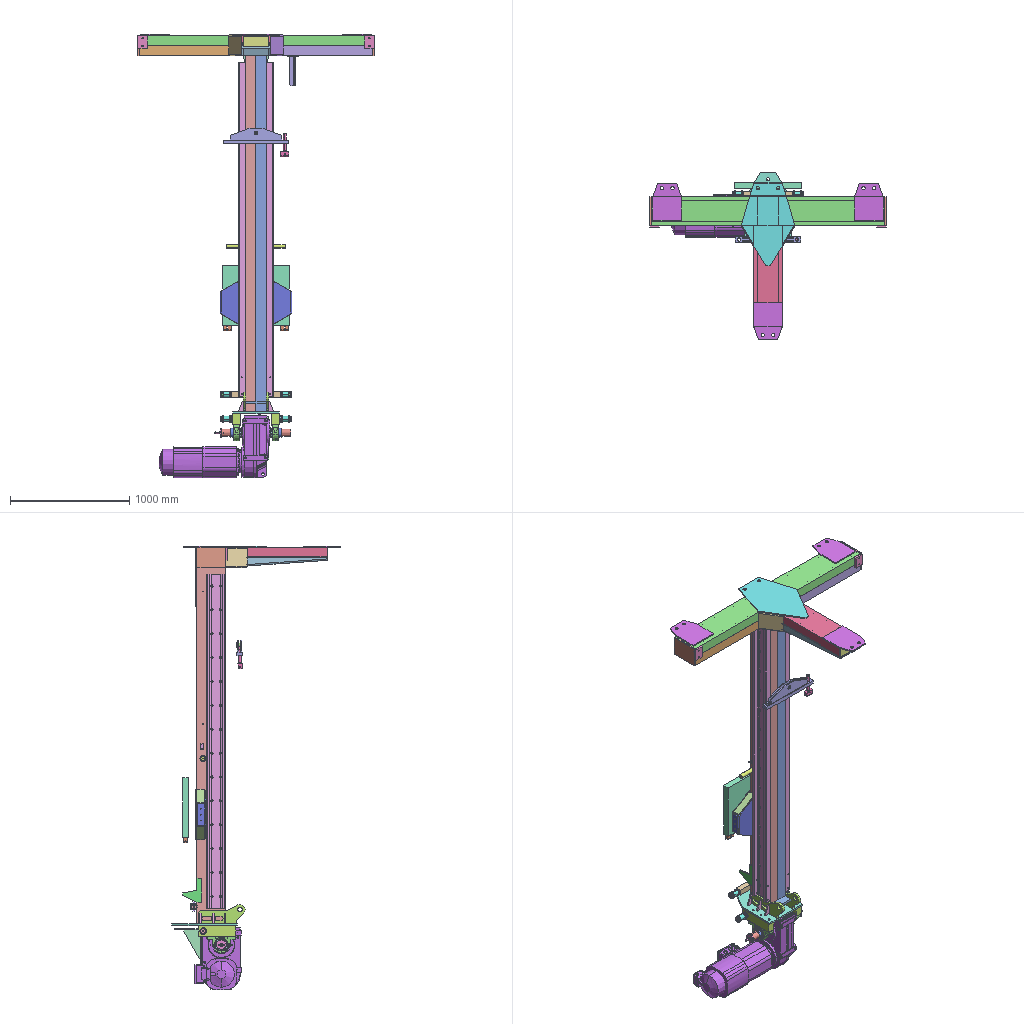Assembly | SolidWorks | 80 different items | 131 placed | box 1980 x 1410 x 3719 mm
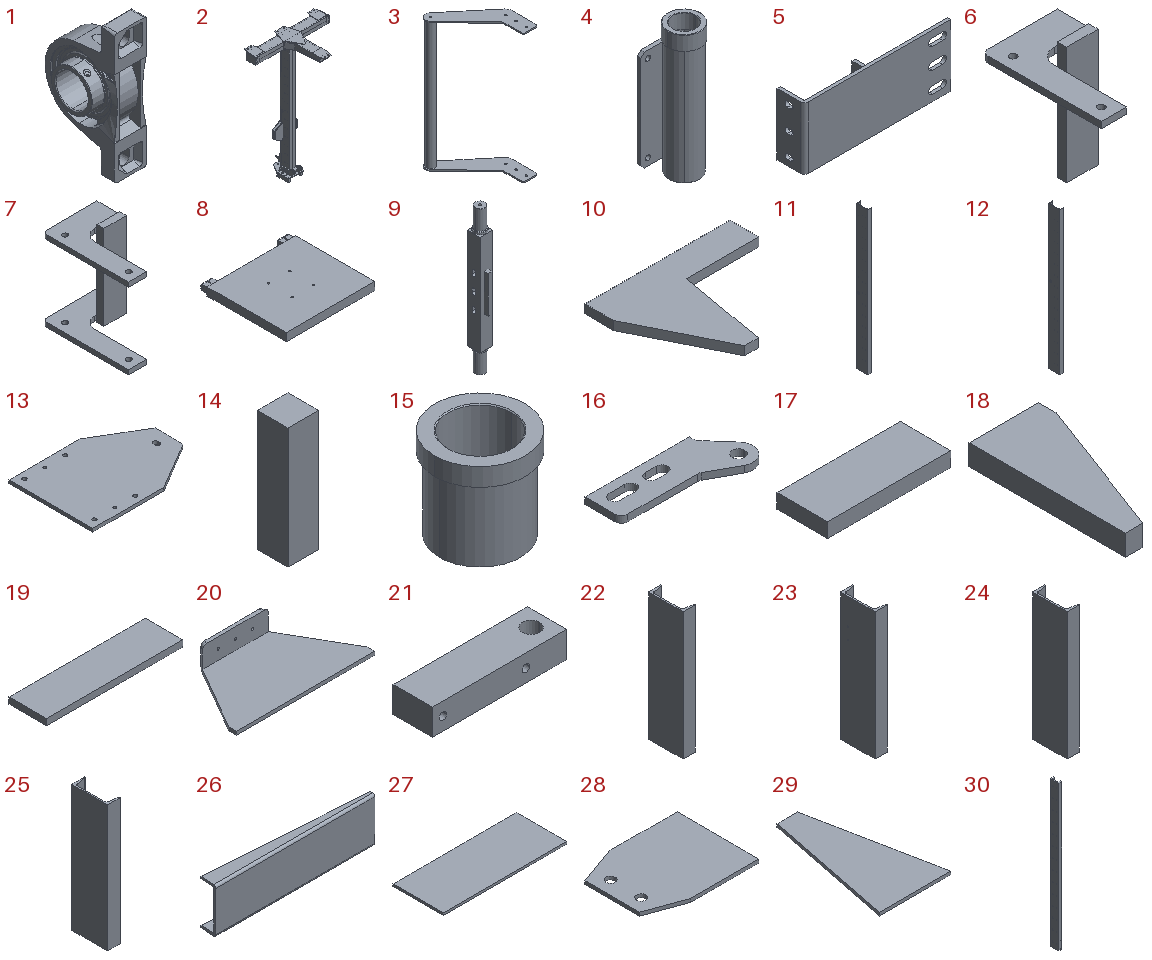Parts list (item | name | quantity | parent item | size | volume | features):
1 | (subassembly) | x2 | - | 69.7 x 138 x 240 mm | 620717 mm3 | features AEMSimFeature 1
2 | (subassembly) | x1 | - | 1980 x 1410 x 3270 mm | 66085382 mm3 | features CompositeCurve 1
3 | (subassembly) | x1 | - | 250 x 320 x 630 mm | 534838 mm3 | features CompositeCurve 1
4 | (subassembly) | x1 | - | 61.848 x 48.7 x 180 mm | 106220 mm3 | -
5 | (subassembly) | x1 | - | 355 x 66 x 150 mm | 497047 mm3 | -
6 | (subassembly) | x1 | - | 120 x 190 x 187 mm | 255476 mm3 | -
7 | (subassembly) | x1 | - | 120 x 190 x 187 mm | 370702 mm3 | -
8 | (subassembly) | x1 | - | 560 x 545 x 50 mm | 14151819 mm3 | -
9 | (subassembly) | x1 | - | 50 x 82 x 584.5 mm | 1278079 mm3 | -
10 | - | x2 | in 2 | 200 x 160 x 12 mm | 181680 mm3 | features Extrusion 1, ICE 1
11 | - | x1 | in 2 | 85 x 240 x 2985 mm | 12447040 mm3 | features HoleWzd 4, Extrusion 1, ICE 1
12 | - | x1 | in 2 | 85 x 240 x 2985 mm | 12447413 mm3 | features HoleWzd 3, Extrusion 1, ICE 1
13 | - | x1 | in 2 | 550 x 390 x 15 mm | 2762557 mm3 | features Extrusion 1, ICE 1
14 | - | x1 | - | 15 x 15 x 60 mm | 13500 mm3 | features Extrusion 1
15 | - | x2 | in 2 | 50 x 50 x 50 mm | 35133 mm3 | features ICE 2, Chamfer 1, Extrusion 1
16 | - | x2 | in 2 | 389 x 164 x 20 mm | 749455 mm3 | features Extrusion 1
17 | - | x1 | in 2 | 170 x 70 x 20 mm | 238000 mm3 | features Extrusion 1
18 | - | x6 | in 2 | 40 x 90 x 12 mm | 28800 mm3 | features MBimport 1
19 | - | x1 | - | 218.3 x 60 x 10 mm | 130980 mm3 | features Extrusion 1
20 | - | x2 | in 2 | 404 x 215 x 70 mm | 757292 mm3 | features ICE 2, Extrusion 1, Fillet 1, HoleWzd 1, Shell 1
21 | - | x2 | in 2 | 310 x 90 x 60 mm | 1555190 mm3 | features ICE 2, Extrusion 1, HoleWzd 1
22 | - | x1 | in 2 | 85 x 240 x 895 mm | 3741522 mm3 | features Extrusion 1, HoleWzd 1
23 | - | x1 | in 2 | 85 x 240 x 895 mm | 3740833 mm3 | features HoleWzd 2, Extrusion 1
24 | - | x2 | in 2 | 85 x 240 x 895 mm | 3742139 mm3 | features Extrusion 1
25 | - | x1 | in 2 | 85 x 240 x 850 mm | 3553986 mm3 | features Extrusion 1
26 | - | x1 | in 2 | 856 x 85 x 240 mm | 3296184 mm3 | features ICE 4, Fillet 2, Extrusion 1, Shell 1
27 | - | x1 | in 2 | 217 x 88 x 4 mm | 76384 mm3 | features Extrusion 1
28 | - | x3 | in 2 | 310 x 240 x 10 mm | 688549 mm3 | features Extrusion 1, ICE 1
29 | - | x1 | in 2 | 280 x 500 x 12 mm | 1080000 mm3 | features Extrusion 1, ICE 1
30 | - | x1 | - | 61.2 x 157.2 x 2800 mm | 12681386 mm3 | features Fillet 2, ICE 2, Extrusion 1, HoleWzd 1
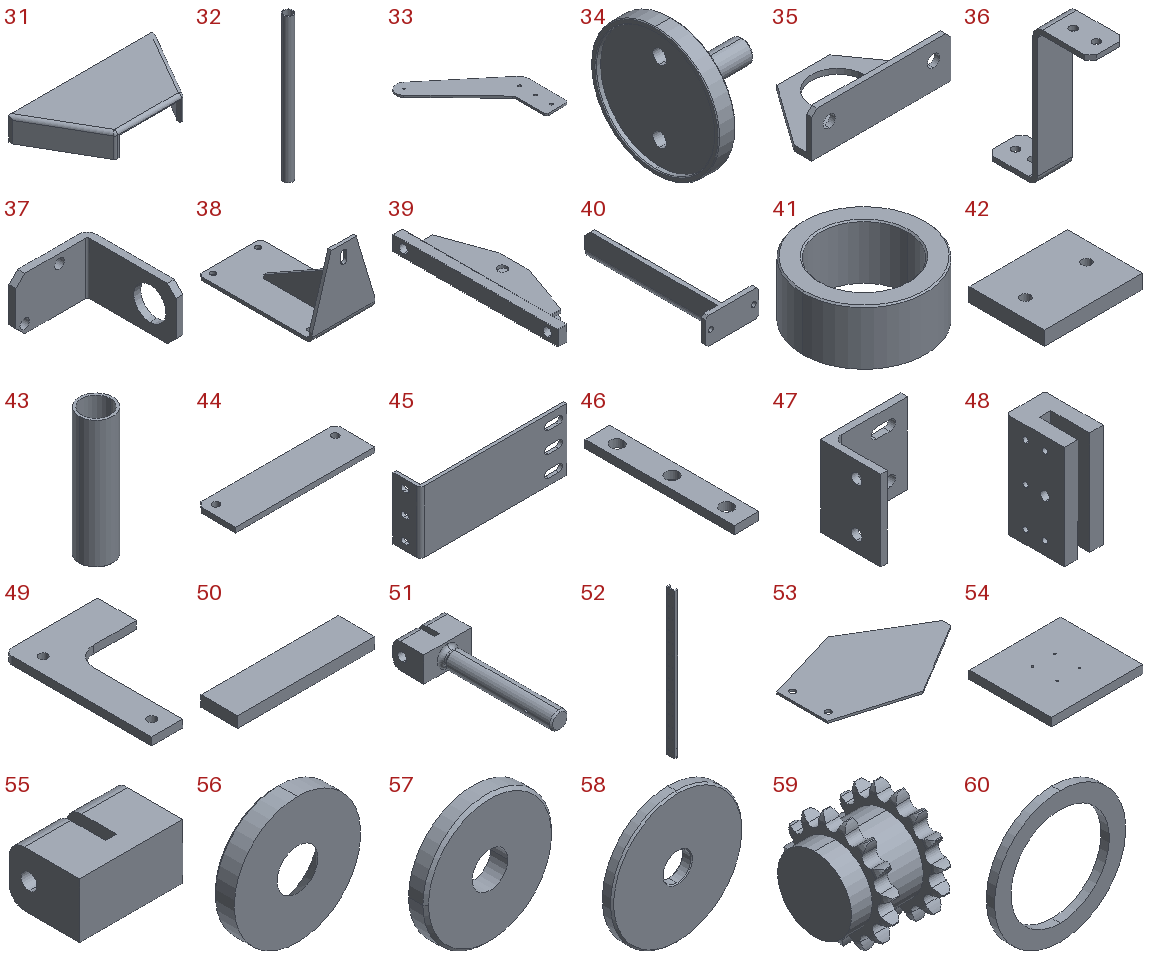31 | - | x2 | in 2 | 424 x 203 x 70 mm | 1081632 mm3 | features ICE 4, Fillet 2, Extrusion 1, Shell 1
32 | - | x1 | - | 40 x 40 x 618 mm | 228632 mm3 | features Extrusion 1, Shell 1
33 | - | x1 | - | 250 x 320 x 6 mm | 153103 mm3 | features Chamfer 1, Extrusion 1
34 | - | x1 | - | 55 x 80 x 80 mm | 48487 mm3 | features MBimport 1
35 | - | x1 | - | 80 x 45 x 25 mm | 11005 mm3 | features MBimport 1
36 | - | x1 | - | 30 x 90 x 120 mm | 23371 mm3 | features MBimport 1
37 | - | x1 | - | 45 x 55 x 30 mm | 9900 mm3 | features ICE 2, Chamfer 1, Extrusion 1
38 | - | x1 | - | 200 x 365 x 230 mm | 1205759 mm3 | features Chamfer 1, MBimport 1
39 | - | x1 | - | 130 x 550 x 50 mm | 1435918 mm3 | features MBimport 1
40 | - | x1 | - | 100 x 255 x 50 mm | 209397 mm3 | features MBimport 1
41 | - | x1 | - | 45 x 45 x 20 mm | 15693 mm3 | features Chamfer 2, Extrusion 1, ICE 1
42 | - | x2 | in 2 | 105 x 80 x 15 mm | 123549 mm3 | features Extrusion 1, HoleWzd 1
43 | - | x1 | - | 42.4 x 42.4 x 160 mm | 63037 mm3 | features Chamfer 1, Extrusion 1, Shell 1
44 | - | x1 | - | 140 x 40 x 5 mm | 27490 mm3 | features Chamfer 1, Extrusion 1, ICE 1
45 | - | x1 | - | 355 x 66 x 150 mm | 470233 mm3 | features ICE 2, Extrusion 1
46 | - | x1 | - | 25 x 150 x 8 mm | 26814 mm3 | features Extrusion 1
47 | - | x1 | - | 100 x 75 x 100 mm | 127963 mm3 | features ICE 2, Extrusion 1, Fillet 1
48 | - | x1 | - | 30 x 45 x 80 mm | 84187 mm3 | features HoleWzd 4, Chamfer 1, Extrusion 1
49 | - | x1 | - | 120 x 190 x 10 mm | 115226 mm3 | features MBimport 1
50 | - | x1 | - | 187 x 50 x 15 mm | 140250 mm3 | features Extrusion 1
51 | - | x1 | - | 65.4 x 197.7 x 35 mm | 150563 mm3 | features MBimport 1
52 | - | x2 | - | 61.2 x 157.2 x 2800 mm | 12681386 mm3 | features Fillet 2, ICE 2, Extrusion 1, HoleWzd 1
53 | - | x1 | in 2 | 690 x 450 x 10 mm | 2029049 mm3 | features Extrusion 1, ICE 1
54 | - | x1 | in 8 | 560 x 500 x 50 mm | 13976046 mm3 | features Extrusion 1, HoleWzd 1, ICE 1
55 | - | x2 | in 8 | 65.4 x 45 x 35 mm | 87886 mm3 | features ICE 2, Extrusion 1, Fillet 1
56 | - | x1 | - | 40 x 7 x 40 mm | 6446 mm3 | features MBimport 1
57 | - | x4 | - | 45 x 6 x 45 mm | 8737 mm3 | features MBimport 1
58 | - | x1 | - | 80 x 6.002 x 80 mm | 28670 mm3 | features Chamfer 1, MBimport 1, MoveFace 1
59 | - | x1 | - | 67.004 x 85.388 x 85.616 mm | 208650 mm3 | features ICE 8, MoveFace 6, HoleWzd 2, BaseBody 1, Chamfer 1
60 | - | x1 | - | 40 x 2.5 x 40 mm | 1374 mm3 | features MBimport 1
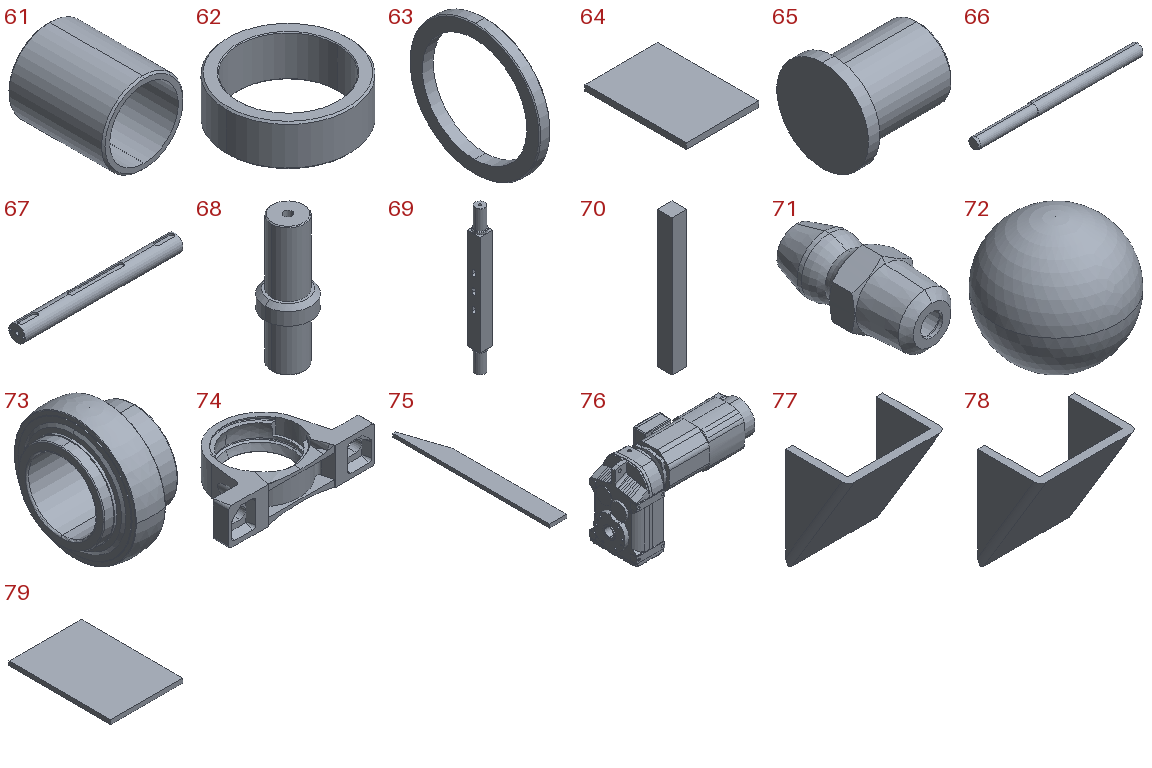61 | - | x4 | - | 47.5 x 56 x 47.5 mm | 28716 mm3 | features MBimport 1
62 | - | x2 | - | 75 x 75 x 25 mm | 39480 mm3 | features MBimport 1
63 | - | x2 | - | 6.3 x 75 x 75 mm | 9961 mm3 | features MBimport 1
64 | - | x1 | - | 151 x 209 x 12 mm | 378708 mm3 | features Extrusion 1
65 | - | x1 | - | 42 x 40 x 40 mm | 30182 mm3 | features MBimport 1
66 | - | x1 | - | 500 x 35 x 35 mm | 451710 mm3 | features MBimport 1
67 | - | x1 | - | 584 x 60 x 60 mm | 1598343 mm3 | features MBimport 1
68 | - | x2 | - | 56 x 56 x 157.5 mm | 215391 mm3 | features Chamfer 2, HoleWzd 2, ICE 2, Extrusion 1
69 | - | x1 | in 9 | 50 x 50 x 584.5 mm | 1201279 mm3 | features ICE 5, Chamfer 3, HoleWzd 2, Extrusion 1
70 | - | x2 | in 9 | 16 x 16 x 150 mm | 38400 mm3 | features Extrusion 1
71 | - | x2 | in 1 | 7.001 x 16.4 x 8.083 mm | 360.824 mm3 | features BaseBody 1
72 | - | x20 | in 1 | 15.875 x 15.875 x 15.875 mm | 2095 mm3 | features BaseBody 1
73 | - | x2 | in 1 | 65.1 x 110 x 110 mm | 162479 mm3 | features BaseBody 1
74 | - | x2 | in 1 | 240 x 138 x 60 mm | 436928 mm3 | features BaseBody 1
75 | - | x1 | - | 60 x 550 x 12 mm | 351000 mm3 | features Extrusion 1, ICE 1
76 | - | x1 | - | 932 x 393 x 531.376 mm | 69762381 mm3 | features BaseBody 1
77 | - | x1 | in 2 | 170 x 110 x 183 mm | 582886 mm3 | features Extrusion 1, Fillet 1, ICE 1, Shell 1
78 | - | x1 | in 2 | 170 x 110 x 183 mm | 582886 mm3 | features Extrusion 1, Fillet 1, ICE 1, Shell 1
79 | - | x2 | in 2 | 170 x 240 x 10 mm | 408000 mm3 | features Extrusion 1
80 | plain washers for clevis pins gb | x1 | - | - | - | -
Mates (type | each side: item.copy, entity, surface, feature):
In the top assembly
Coincident | 11.1 face plane Boss-Extrude 1 | 52.1 face plane Boss-Extrude 1
Concentric | 11.1 face cylinder M10 Tapped Hole 2 | 52.1 face cylinder Cut-Extrude 2 | 2 times
Coincident | 12.1 face plane Boss-Extrude 1 | 52.2 face plane Boss-Extrude 1
Coincident | 52.1 face plane Boss-Extrude 1 | 52.2 face plane Boss-Extrude 1 | 2 times
Coincident | 48.1 face plane Boss-Extrude 1 | 40.1 face plane 526914D.STEP | 2 times
Coincident | 48.1 face plane Boss-Extrude 1 | 35.1 face plane 521957D.STEP
Concentric | 48.1 face cylinder M5 Tapped Hole 1 | 35.1 face cylinder 521957D.STEP | 2 times
Coincident | 23.1 face plane Boss-Extrude 1 | 40.1 face plane 526914D.STEP
Concentric | 23.1 face cylinder M8 Tapped Hole 1 | 40.1 face cylinder 526914D.STEP | 2 times
Coincident | 21.1 face plane Boss-Extrude 1 | 74.1 face plane housingSY 512 M-h(1)
Slot | 74.1 face cylinder housingSY 512 M-h(1) | 21.1 face cylinder Cut-Extrude 1 | 2 times
Coincident | 21.2 face plane Boss-Extrude 1 | 74.2 face plane housingSY 512 M-h(1)
Slot | 74.2 face cylinder housingSY 512 M-h(1) | 21.2 face cylinder Cut-Extrude 1 | 2 times
Concentric | 73.1 face cylinder YAR 212-2F-75.64103002212-b(1) | 76.1 face cylinder Input 1
Width | 76.1 face plane Input 1 | 76.1 face plane Input 1 | 21.1 face plane Boss-Extrude 1 | 21.2 face plane Boss-Extrude 1
Coincident | 76.1 face plane Input 1 | 38.1 face plane 526597D.STEP
Concentric | 76.1 face cylinder Input 1 | 38.1 face cylinder 526597D.STEP | 2 times
Concentric | 73.1 face cylinder YAR 212-2F-75.64103002212-b(1) | 67.1 face cylinder 741959D.STEP
Parallel | 11.1 face plane Boss-Extrude 1 | 67.1 face plane 741959D.STEP
Width | 67.1 face plane 741959D.STEP | 67.1 face plane 741959D.STEP | 76.1 face plane Input 1 | 76.1 face plane Input 1
Concentric | 67.1 face cylinder 741959D.STEP | 62.1 face cylinder 732089D.STEP
Coincident | 73.2 face plane YAR 212-2F-75.64103002212-b(1) | 62.1 face plane 732089D.STEP
Concentric | 67.1 face cylinder 741959D.STEP | 62.2 face cylinder 732089D.STEP
Coincident | 73.1 face plane YAR 212-2F-75.64103002212-b(1) | 62.2 face plane 732089D.STEP
Concentric | 67.1 face cylinder 741959D.STEP | 63.1 face cylinder 732090D.STEP
Coincident | 76.1 face plane Input 1 | 63.1 face plane 732090D.STEP
Concentric | 67.1 face cylinder 741959D.STEP | 63.2 face cylinder 732090D.STEP
Coincident | 76.1 face plane Input 1 | 63.2 face plane 732090D.STEP
Coincident | 67.1 face plane 741959D.STEP | 34.1 face plane 513942D.STEP
Concentric | 67.1 edge | 34.1 face cylinder 513942D.STEP
Concentric | 67.1 face cylinder 741959D.STEP | 34.1 face cylinder 513942D.STEP
Coincident | 12.1 face plane Boss-Extrude 1 | 69.1 face plane Boss-Extrude 3
Slot | 69.1 face plane Cut-Extrude 1 | 11.1 face cylinder M12 Tapped Hole 1
Slot | 69.1 face plane Cut-Extrude 1 | 12.1 face cylinder M12 Tapped Hole 1
Concentric | 61.1 face cylinder 732088D.STEP | 69.1 face cylinder Boss-Extrude 1
Concentric | 69.1 face cylinder Boss-Extrude 5 | 61.2 face cylinder 732088D.STEP
Coincident | 69.1 face plane Boss-Extrude 1 | 57.1 face plane 571148D.STEP
Concentric | 69.1 face cylinder Boss-Extrude 1 | 57.1 face cylinder 571148D.STEP
Coincident | 69.1 face plane Boss-Extrude 5 | 57.2 face plane 571148D.STEP
Concentric | 61.2 face cylinder 732088D.STEP | 57.2 face cylinder 571148D.STEP
Concentric | 21.1 face cylinder Cut-Extrude 2 | 68.1 face cylinder Boss-Extrude 1
Coincident | 21.1 face plane Boss-Extrude 1 | 68.1 face plane Boss-Extrude 2
Concentric | 21.2 face cylinder Cut-Extrude 2 | 68.2 face cylinder Boss-Extrude 1
Coincident | 21.2 face plane Boss-Extrude 1 | 68.2 face plane Boss-Extrude 2
Concentric | 68.1 face cylinder Boss-Extrude 3 | 61.3 face cylinder 732088D.STEP
Concentric | 68.2 face cylinder Boss-Extrude 3 | 61.4 face cylinder 732088D.STEP
Parallel | 13.1 face plane Boss-Extrude 1 | 38.1 face plane 526597D.STEP
Coincident | 68.2 face plane Boss-Extrude 3 | 57.3 face plane 571148D.STEP
Concentric | 68.2 face cylinder Boss-Extrude 3 | 57.3 face cylinder 571148D.STEP
Coincident | 68.1 face plane Boss-Extrude 3 | 57.4 face plane 571148D.STEP
Concentric | 68.1 face cylinder Boss-Extrude 3 | 57.4 face cylinder 571148D.STEP
Concentric | 15.1 face cylinder Cut-Extrude 1 | 66.1 face cylinder 741958D.STEP
Width | 66.1 face plane 741958D.STEP | 66.1 face plane 741958D.STEP | 11.1 face plane Boss-Extrude 1 | 12.1 face plane Boss-Extrude 1
Coincident | 11.1 face plane Boss-Extrude 1 | 37.1 face plane Boss-Extrude 1
Parallel | 11.1 face plane Boss-Extrude 1 | 37.1 face plane Boss-Extrude 1
Parallel | 12.1 face plane Boss-Extrude 1 | 54.1 face plane Boss-Extrude 1
Width | 54.1 face plane Boss-Extrude 1 | 54.1 face plane Boss-Extrude 1 | 11.1 face plane Boss-Extrude 1 | 12.1 face plane Boss-Extrude 1
Lock | 11.1 select_type:0 | 54.1 select_type:0
Concentric | 39.1 face cylinder 526627D.STEP | 65.1 face cylinder 740793D.STEP
Coincident | 39.1 face plane 526627D.STEP | 65.1 face plane 740793D.STEP
Concentric | 39.1 face cylinder 526627D.STEP | 51.1 face cylinder 546779D.STEP
Parallel | 39.1 face plane 526627D.STEP | 51.1 face plane 546779D.STEP
Lock | 39.1 select_type:0 | 51.1 select_type:0
Width | 39.1 face plane 526627D.STEP | 39.1 face plane 526627D.STEP | 52.2 face plane Boss-Extrude 1 | 52.1 face plane Boss-Extrude 1
Lock | 52.1 select_type:0 | 39.1 select_type:0
In subassembly 2
Coincident | 11.2 face plane Boss-Extrude 1 | 12.2 face plane Boss-Extrude 1 | 3 times
Coincident | 12.2 face plane Boss-Extrude 1 | 16.1 face plane Boss-Extrude 2 | 2 times
Coincident | 11.2 face plane Boss-Extrude 1 | 16.2 face plane Boss-Extrude 2
Coincident | 16.1 face plane Boss-Extrude 2 | 16.2 face plane Boss-Extrude 2 | 2 times
Coincident | 16.1 face plane Boss-Extrude 2 | 18.1 face plane 507728D24.STEP
Coincident | 16.1 face plane Boss-Extrude 2 | 18.2 face plane 507728D24.STEP
Coincident | 18.1 face plane 507728D24.STEP | 18.3 face plane 507728D24.STEP | 2 times
Coincident | 18.4 face plane 507728D24.STEP | 18.5 face plane 507728D24.STEP | 2 times
Coincident | 18.6 face plane 507728D24.STEP | 18.4 face plane 507728D24.STEP | 2 times
Coincident | 16.2 face plane Boss-Extrude 2 | 18.5 face plane 507728D24.STEP
Coincident | 18.2 face plane 507728D24.STEP | 18.6 face plane 507728D24.STEP
Coincident | 18.3 face plane 507728D24.STEP | 18.5 face plane 507728D24.STEP
Coincident | 18.1 face plane 507728D24.STEP | 18.4 face plane 507728D24.STEP
Coincident | 12.2 face plane Boss-Extrude 1 | 13.2 face plane Boss-Extrude 1
Width | 13.2 face plane Boss-Extrude 1 | 13.2 face plane Boss-Extrude 1 | 11.2 face plane Boss-Extrude 1 | 12.2 face plane Boss-Extrude 1
Coincident | 18.3 face plane 507728D24.STEP | 13.2 face plane Boss-Extrude 1
Coincident | 18.1 face plane 507728D24.STEP | 18.2 face plane 507728D24.STEP
DistanceDim | 18.1 face plane 507728D24.STEP | 18.2 face plane 507728D24.STEP
DistanceDim | 18.1 face plane 507728D24.STEP | 18.3 face plane 507728D24.STEP
DistanceDim | 16.1 face plane Boss-Extrude 2 | 18.2 face plane 507728D24.STEP
DistanceDim | 16.1 face plane Boss-Extrude 2 | 12.2 face plane Boss-Extrude 1
Coincident | 12.2 face plane Boss-Extrude 1 | 22.1 face plane Boss-Extrude 1 | 2 times
Coincident | 12.2 face plane Boss-Extrude 1 | 23.2 face plane Boss-Extrude 1 | 2 times
DistanceDim | 22.1 face plane Boss-Extrude 1 | 23.2 face plane Boss-Extrude 1
Width | 23.2 face plane Boss-Extrude 1 | 22.1 face plane Boss-Extrude 1 | 11.2 face plane Boss-Extrude 1 | 12.2 face plane Boss-Extrude 1
Coincident | 12.2 face plane Boss-Extrude 1 | 24.1 face plane Boss-Extrude 1
Coincident | 23.2 face plane Boss-Extrude 1 | 24.1 face plane Boss-Extrude 1 | 2 times
Coincident | 24.1 face plane Boss-Extrude 1 | 24.2 face plane Boss-Extrude 1
Coincident | 22.1 face plane Boss-Extrude 1 | 24.2 face plane Boss-Extrude 1 | 2 times
Coincident | 24.1 face plane Boss-Extrude 1 | 25.1 face plane Boss-Extrude 1 | 2 times
DistanceDim | 25.1 face plane Boss-Extrude 1 | 24.1 face plane Boss-Extrude 1
Coincident | 25.1 face plane Boss-Extrude 1 | 26.1 face plane Cut-Extrude 1
Coincident | 22.1 face plane Boss-Extrude 1 | 26.1 face plane Boss-Extrude 2
Coincident | 25.1 face plane Boss-Extrude 1 | 26.1 face plane Boss-Extrude 1
Coincident | 25.1 face plane Boss-Extrude 1 | 27.1 face plane Boss-Extrude 1 | 2 times
Width | 27.1 face plane Boss-Extrude 1 | 27.1 face plane Boss-Extrude 1 | 25.1 face plane Boss-Extrude 1 | 25.1 face plane Boss-Extrude 1
Coincident | 25.1 face plane Boss-Extrude 1 | 28.1 face plane Boss-Extrude 1
Width | 25.1 face plane Boss-Extrude 1 | 25.1 face plane Boss-Extrude 1 | 28.1 face plane Boss-Extrude 1 | 28.1 face plane Boss-Extrude 1
DistanceDim | 28.1 face plane Boss-Extrude 1 | 27.1 face plane Boss-Extrude 1
Coincident | 28.2 face plane Boss-Extrude 1 | 28.3 face plane Boss-Extrude 1 | 2 times
Coincident | 24.1 face plane Boss-Extrude 1 | 28.3 face plane Boss-Extrude 1
DistanceDim | 28.3 face plane Boss-Extrude 1 | 24.1 face plane Boss-Extrude 1
DistanceDim | 28.2 face plane Boss-Extrude 1 | 24.2 face plane Boss-Extrude 1
DistanceDim | 24.1 face plane Boss-Extrude 1 | 28.3 face plane Boss-Extrude 1
Coincident | 12.2 face plane Boss-Extrude 1 | 29.1 face plane Boss-Extrude 1
Coincident | 24.2 face plane Boss-Extrude 1 | 29.1 face plane Boss-Extrude 1
Width | 29.1 face plane Cut-Extrude 1 | 29.1 face plane Cut-Extrude 1 | 12.2 face plane Boss-Extrude 1 | 11.2 face plane Boss-Extrude 1
Coincident | 22.1 face plane Boss-Extrude 1 | 79.1 face plane Boss-Extrude 1 | 3 times
Coincident | 23.2 face plane Boss-Extrude 1 | 79.2 face plane Boss-Extrude 1 | 3 times
Coincident | 20.1 face plane Boss-Extrude 1 | 31.1 face plane Boss-Extrude 3
Width | 20.1 face plane Cut-Extrude 1 | 20.1 face plane Cut-Extrude 1 | 31.1 face plane Cut-Extrude 1 | 31.1 face plane Cut-Extrude 1
DistanceDim | 31.1 face plane Boss-Extrude 1 | 11.2 face plane Boss-Extrude 1
DistanceDim | 20.1 face plane Boss-Extrude 1 | 28.2 face plane Boss-Extrude 1
Coincident | 31.2 face plane Boss-Extrude 3 | 20.2 face plane Boss-Extrude 1
Coincident | 31.2 face plane Boss-Extrude 1 | 20.2 face plane Shell 1
Width | 31.2 face plane Cut-Extrude 1 | 31.2 face plane Cut-Extrude 1 | 20.2 face plane Cut-Extrude 1 | 20.2 face plane Cut-Extrude 1
Coincident | 12.2 face plane Boss-Extrude 1 | 20.2 face plane Boss-Extrude 1
DistanceDim | 31.2 face plane Boss-Extrude 1 | 12.2 face plane Boss-Extrude 1
DistanceDim | 20.2 face plane Boss-Extrude 1 | 28.3 face plane Boss-Extrude 1
Coincident | 20.1 face plane Shell 1 | 31.1 face plane Boss-Extrude 1
Coincident | 11.2 face plane Boss-Extrude 1 | 20.1 face plane Boss-Extrude 1
Coincident | 24.2 face plane Boss-Extrude 1 | 42.1 face plane Boss-Extrude 1
Coincident | 79.1 face plane Boss-Extrude 1 | 42.1 face plane Boss-Extrude 1
DistanceDim | 42.1 face plane Boss-Extrude 1 | 24.2 face plane Boss-Extrude 1
Coincident | 42.1 face plane Boss-Extrude 1 | 42.2 face plane Boss-Extrude 1 | 2 times
Coincident | 79.2 face plane Boss-Extrude 1 | 42.2 face plane Boss-Extrude 1
Coincident | 24.1 face plane Boss-Extrude 1 | 78.1 face plane Cut-Extrude 3
Coincident | 25.1 face plane Boss-Extrude 1 | 78.1 face plane Boss-Extrude 2 | 2 times
Coincident | 24.2 face plane Boss-Extrude 1 | 77.1 face plane Cut-Extrude 3
Coincident | 25.1 face plane Boss-Extrude 1 | 77.1 face plane Boss-Extrude 2 | 2 times
Coincident | 25.1 face plane Boss-Extrude 1 | 53.1 face plane Boss-Extrude 1
Parallel | 24.1 face plane Boss-Extrude 1 | 53.1 face plane Boss-Extrude 1
Width | 53.1 face plane Cut-Extrude 1 | 53.1 face plane Cut-Extrude 1 | 25.1 face plane Boss-Extrude 1 | 25.1 face plane Boss-Extrude 1
DistanceDim | 53.1 face plane Boss-Extrude 1 | 24.1 face plane Boss-Extrude 1
Coincident | 11.2 face plane Boss-Extrude 1 | 10.1 face plane Boss-Extrude 1
Coincident | 10.1 face plane Boss-Extrude 1 | 10.2 face plane Boss-Extrude 1 | 2 times
DistanceDim | 10.2 face plane Boss-Extrude 1 | 13.2 face plane Boss-Extrude 1
Coincident | 12.2 face plane Boss-Extrude 1 | 10.2 face plane Boss-Extrude 1
Coincident | 12.2 face plane Boss-Extrude 1 | 10.2 face plane Cut-Extrude 1
Concentric | 11.2 face cylinder Cut-Extrude 1 | 15.2 face cylinder Boss-Extrude 2
Coincident | 11.2 face plane Boss-Extrude 1 | 15.2 face plane Boss-Extrude 1
Concentric | 12.2 face cylinder Cut-Extrude 1 | 15.3 face cylinder Boss-Extrude 2
Coincident | 12.2 face plane Boss-Extrude 1 | 15.3 face plane Boss-Extrude 1
Coincident | 16.2 face plane Boss-Extrude 2 | 17.1 face plane Boss-Extrude 1
Coincident | 18.3 face plane 507728D24.STEP | 17.1 face plane Boss-Extrude 1
Coincident | 12.2 face plane Boss-Extrude 1 | 17.1 face plane Boss-Extrude 1
Coincident | 13.2 face plane Boss-Extrude 1 | 21.3 face plane Boss-Extrude 1
Parallel | 13.2 face cylinder Cut-Extrude 1 | 21.3 face cylinder Cut-Extrude 1
Coincident | 13.2 edge | 21.3 face cylinder Cut-Extrude 1
Concentric | 13.2 face cylinder Cut-Extrude 1 | 21.3 face cylinder Cut-Extrude 1
Coincident | 21.3 face plane Boss-Extrude 1 | 21.4 face plane Boss-Extrude 1 | 2 times
Concentric | 13.2 face cylinder Cut-Extrude 1 | 21.4 face cylinder Cut-Extrude 1
DistanceDim | 13.2 face plane Boss-Extrude 1 | 18.5 face plane 507728D24.STEP
In subassembly 9
Coincident | 70.1 face plane Boss-Extrude 1 | 70.2 face plane Boss-Extrude 1 | 2 times
Coincident | 69.2 face plane Boss-Extrude 3 | 70.2 face plane Boss-Extrude 1
Coincident | 69.2 face plane Boss-Extrude 3 | 70.1 face plane Boss-Extrude 1
Width | 70.1 face plane Boss-Extrude 1 | 70.1 face plane Boss-Extrude 1 | 69.2 face plane Boss-Extrude 3 | 69.2 face plane Boss-Extrude 3 | 2 times
In subassembly 8
Coincident | 54.2 face plane Boss-Extrude 1 | 55.1 face plane Boss-Extrude 1
Coincident | 55.2 face plane Boss-Extrude 1 | 55.1 face plane Boss-Extrude 1 | 2 times
DistanceDim | 55.1 face plane Boss-Extrude 1 | 55.2 face plane Boss-Extrude 1
DistanceDim | 55.1 face plane Boss-Extrude 1 | 54.2 face plane Boss-Extrude 1
DistanceDim | 55.2 face plane Boss-Extrude 1 | 54.2 face plane Boss-Extrude 1